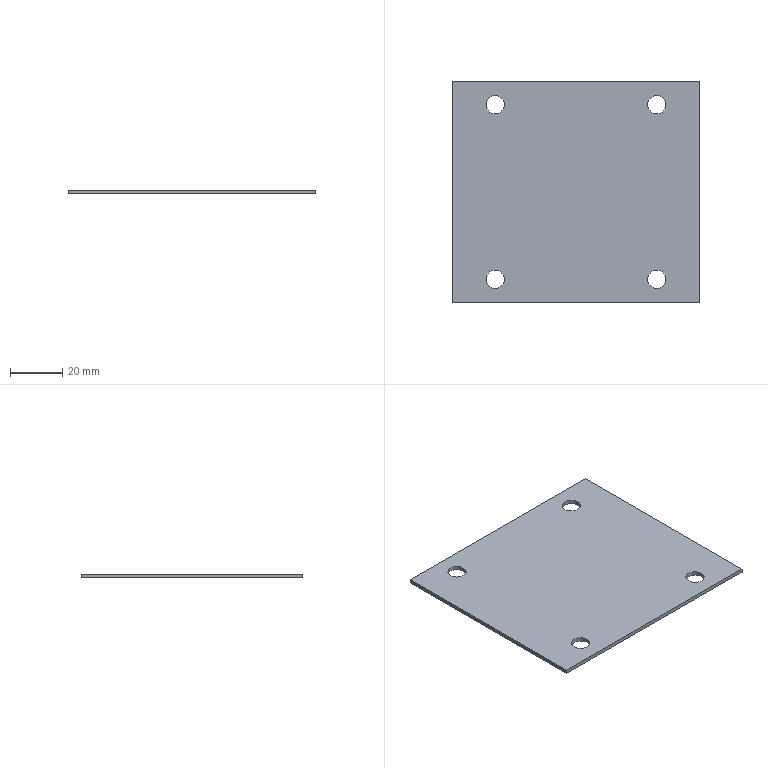Part | STEP file | GLSJ-10-46 | 1 solid | 14 faces | box 95 x 85 x 1.5 mm | volume 11882 mm3 | cylinder 8 | plane 6 | commonest cylinder face diameters 7 x8
STEP:
#1=CARTESIAN_POINT('',(0.,0.,0.));
#2=DIRECTION('',(0.,0.,1.));
#3=DIRECTION('',(1.,0.,0.));
#4=AXIS2_PLACEMENT_3D('',#1,#2,#3);
#5=CARTESIAN_POINT('',(-27.5,-33.5,0.));
#6=VERTEX_POINT('',#5);
#7=CARTESIAN_POINT('',(-27.5,-33.5,1.5));
#8=VERTEX_POINT('',#7);
#9=CARTESIAN_POINT('',(-27.5,-33.5,0.));
#10=DIRECTION('',(0.,0.,1.));
#11=VECTOR('',#10,1.);
#12=LINE('',#9,#11);
#13=CARTESIAN_POINT('',(-31.,-33.5,0.));
#14=DIRECTION('',(0.,0.,1.));
#15=DIRECTION('',(1.,0.,0.));
#16=AXIS2_PLACEMENT_3D('',#13,#14,#15);
#17=CYLINDRICAL_SURFACE('',#16,3.5);
#18=CARTESIAN_POINT('',(6.283,0.));
#19=DIRECTION('',(0.,1.));
#20=VECTOR('',#19,1.);
#21=LINE('',#18,#20);
#22=(GEOMETRIC_REPRESENTATION_CONTEXT(2)PARAMETRIC_REPRESENTATION_CONTEXT()REPRESENTATION_CONTEXT('',''));
#23=DEFINITIONAL_REPRESENTATION('',(#21),#22);
#24=PCURVE('',#17,#23);
#25=CARTESIAN_POINT('',(-31.,-33.5,0.));
#26=DIRECTION('',(0.,0.,1.));
#27=DIRECTION('',(1.,0.,0.));
#28=AXIS2_PLACEMENT_3D('',#25,#26,#27);
#29=CYLINDRICAL_SURFACE('',#28,3.5);
#30=CARTESIAN_POINT('',(0.,0.));
#31=DIRECTION('',(0.,1.));
#32=VECTOR('',#31,1.);
#33=LINE('',#30,#32);
#34=(GEOMETRIC_REPRESENTATION_CONTEXT(2)PARAMETRIC_REPRESENTATION_CONTEXT()REPRESENTATION_CONTEXT('',''));
#35=DEFINITIONAL_REPRESENTATION('',(#33),#34);
#36=PCURVE('',#29,#35);
#37=SURFACE_CURVE('',#12,(#24,#36),.PCURVE_S1.);
#38=EDGE_CURVE('',#6,#8,#37,.T.);
#39=ORIENTED_EDGE('',*,*,#38,.T.);
#40=CARTESIAN_POINT('',(-34.5,-33.5,1.5));
#41=VERTEX_POINT('',#40);
#42=CARTESIAN_POINT('',(-31.,-33.5,1.5));
#43=DIRECTION('',(0.,0.,1.));
#44=DIRECTION('',(-1.,0.,0.));
#45=AXIS2_PLACEMENT_3D('',#42,#43,#44);
#46=CIRCLE('',#45,3.5);
#47=CARTESIAN_POINT('',(3.142,1.5));
#48=DIRECTION('',(1.,0.));
#49=VECTOR('',#48,1.);
#50=LINE('',#47,#49);
#51=(GEOMETRIC_REPRESENTATION_CONTEXT(2)PARAMETRIC_REPRESENTATION_CONTEXT()REPRESENTATION_CONTEXT('',''));
#52=DEFINITIONAL_REPRESENTATION('',(#50),#51);
#53=PCURVE('',#17,#52);
#54=CARTESIAN_POINT('',(0.,0.,1.5));
#55=DIRECTION('',(0.,0.,-1.));
#56=DIRECTION('',(-1.,0.,0.));
#57=AXIS2_PLACEMENT_3D('',#54,#55,#56);
#58=PLANE('',#57);
#59=CARTESIAN_POINT('',(34.5,-33.5));
#60=CARTESIAN_POINT('',(34.5,-39.562));
#61=CARTESIAN_POINT('',(29.25,-36.531));
#62=CARTESIAN_POINT('',(24.,-33.5));
#63=CARTESIAN_POINT('',(29.25,-30.469));
#64=CARTESIAN_POINT('',(34.5,-27.438));
#65=CARTESIAN_POINT('',(34.5,-33.5));
#66=(BOUNDED_CURVE()B_SPLINE_CURVE(2,(#59,#60,#61,#62,#63,#64,#65),.UNSPECIFIED.,.T.,.F.)B_SPLINE_CURVE_WITH_KNOTS((1,2,2,2,2,1),(-2.094,0.,2.094,4.189,6.283,8.378),.UNSPECIFIED.)CURVE()GEOMETRIC_REPRESENTATION_ITEM()RATIONAL_B_SPLINE_CURVE((1.,0.5,1.,0.5,1.,0.5,1.))REPRESENTATION_ITEM(''));
#67=(GEOMETRIC_REPRESENTATION_CONTEXT(2)PARAMETRIC_REPRESENTATION_CONTEXT()REPRESENTATION_CONTEXT('',''));
#68=DEFINITIONAL_REPRESENTATION('',(#66),#67);
#69=PCURVE('',#58,#68);
#70=SURFACE_CURVE('',#46,(#53,#69),.PCURVE_S1.);
#71=EDGE_CURVE('',#41,#8,#70,.T.);
#72=ORIENTED_EDGE('',*,*,#71,.F.);
#73=CARTESIAN_POINT('',(-34.5,-33.5,0.));
#74=VERTEX_POINT('',#73);
#75=CARTESIAN_POINT('',(-34.5,-33.5,0.));
#76=DIRECTION('',(0.,0.,1.));
#77=VECTOR('',#76,1.);
#78=LINE('',#75,#77);
#79=CARTESIAN_POINT('',(3.142,0.));
#80=DIRECTION('',(0.,1.));
#81=VECTOR('',#80,1.);
#82=LINE('',#79,#81);
#83=(GEOMETRIC_REPRESENTATION_CONTEXT(2)PARAMETRIC_REPRESENTATION_CONTEXT()REPRESENTATION_CONTEXT('',''));
#84=DEFINITIONAL_REPRESENTATION('',(#82),#83);
#85=PCURVE('',#17,#84);
#86=CARTESIAN_POINT('',(3.142,0.));
#87=DIRECTION('',(0.,1.));
#88=VECTOR('',#87,1.);
#89=LINE('',#86,#88);
#90=(GEOMETRIC_REPRESENTATION_CONTEXT(2)PARAMETRIC_REPRESENTATION_CONTEXT()REPRESENTATION_CONTEXT('',''));
#91=DEFINITIONAL_REPRESENTATION('',(#89),#90);
#92=PCURVE('',#29,#91);
#93=SURFACE_CURVE('',#78,(#85,#92),.PCURVE_S1.);
#94=EDGE_CURVE('',#74,#41,#93,.T.);
#95=ORIENTED_EDGE('',*,*,#94,.F.);
#96=CARTESIAN_POINT('',(-31.,-33.5,0.));
#97=DIRECTION('',(0.,0.,1.));
#98=DIRECTION('',(-1.,0.,0.));
#99=AXIS2_PLACEMENT_3D('',#96,#97,#98);
#100=CIRCLE('',#99,3.5);
#101=CARTESIAN_POINT('',(3.142,0.));
#102=DIRECTION('',(1.,0.));
#103=VECTOR('',#102,1.);
#104=LINE('',#101,#103);
#105=(GEOMETRIC_REPRESENTATION_CONTEXT(2)PARAMETRIC_REPRESENTATION_CONTEXT()REPRESENTATION_CONTEXT('',''));
#106=DEFINITIONAL_REPRESENTATION('',(#104),#105);
#107=PCURVE('',#17,#106);
#108=CARTESIAN_POINT('',(0.,0.,0.));
#109=DIRECTION('',(0.,0.,-1.));
#110=DIRECTION('',(-1.,0.,0.));
#111=AXIS2_PLACEMENT_3D('',#108,#109,#110);
#112=PLANE('',#111);
#113=CARTESIAN_POINT('',(34.5,-33.5));
#114=CARTESIAN_POINT('',(34.5,-39.562));
#115=CARTESIAN_POINT('',(29.25,-36.531));
#116=CARTESIAN_POINT('',(24.,-33.5));
#117=CARTESIAN_POINT('',(29.25,-30.469));
#118=CARTESIAN_POINT('',(34.5,-27.438));
#119=CARTESIAN_POINT('',(34.5,-33.5));
#120=(BOUNDED_CURVE()B_SPLINE_CURVE(2,(#113,#114,#115,#116,#117,#118,#119),.UNSPECIFIED.,.T.,.F.)B_SPLINE_CURVE_WITH_KNOTS((1,2,2,2,2,1),(-2.094,0.,2.094,4.189,6.283,8.378),.UNSPECIFIED.)CURVE()GEOMETRIC_REPRESENTATION_ITEM()RATIONAL_B_SPLINE_CURVE((1.,0.5,1.,0.5,1.,0.5,1.))REPRESENTATION_ITEM(''));
#121=(GEOMETRIC_REPRESENTATION_CONTEXT(2)PARAMETRIC_REPRESENTATION_CONTEXT()REPRESENTATION_CONTEXT('',''));
#122=DEFINITIONAL_REPRESENTATION('',(#120),#121);
#123=PCURVE('',#112,#122);
#124=SURFACE_CURVE('',#100,(#107,#123),.PCURVE_S1.);
#125=EDGE_CURVE('',#74,#6,#124,.T.);
#126=ORIENTED_EDGE('',*,*,#125,.T.);
#127=EDGE_LOOP('',(#39,#72,#95,#126));
#128=FACE_BOUND('',#127,.F.);
#129=ADVANCED_FACE('',(#128),#17,.F.);
#130=CARTESIAN_POINT('',(34.5,-33.5,0.));
#131=VERTEX_POINT('',#130);
#132=CARTESIAN_POINT('',(34.5,-33.5,1.5));
#133=VERTEX_POINT('',#132);
#134=CARTESIAN_POINT('',(34.5,-33.5,0.));
#135=DIRECTION('',(0.,0.,1.));
#136=VECTOR('',#135,1.);
#137=LINE('',#134,#136);
#138=CARTESIAN_POINT('',(31.,-33.5,0.));
#139=DIRECTION('',(0.,0.,1.));
#140=DIRECTION('',(1.,0.,0.));
#141=AXIS2_PLACEMENT_3D('',#138,#139,#140);
#142=CYLINDRICAL_SURFACE('',#141,3.5);
#143=CARTESIAN_POINT('',(6.283,0.));
#144=DIRECTION('',(0.,1.));
#145=VECTOR('',#144,1.);
#146=LINE('',#143,#145);
#147=(GEOMETRIC_REPRESENTATION_CONTEXT(2)PARAMETRIC_REPRESENTATION_CONTEXT()REPRESENTATION_CONTEXT('',''));
#148=DEFINITIONAL_REPRESENTATION('',(#146),#147);
#149=PCURVE('',#142,#148);
#150=CARTESIAN_POINT('',(31.,-33.5,0.));
#151=DIRECTION('',(0.,0.,1.));
#152=DIRECTION('',(1.,0.,0.));
#153=AXIS2_PLACEMENT_3D('',#150,#151,#152);
#154=CYLINDRICAL_SURFACE('',#153,3.5);
#155=CARTESIAN_POINT('',(0.,0.));
#156=DIRECTION('',(0.,1.));
#157=VECTOR('',#156,1.);
#158=LINE('',#155,#157);
#159=(GEOMETRIC_REPRESENTATION_CONTEXT(2)PARAMETRIC_REPRESENTATION_CONTEXT()REPRESENTATION_CONTEXT('',''));
#160=DEFINITIONAL_REPRESENTATION('',(#158),#159);
#161=PCURVE('',#154,#160);
#162=SURFACE_CURVE('',#137,(#149,#161),.PCURVE_S1.);
#163=EDGE_CURVE('',#131,#133,#162,.T.);
#164=ORIENTED_EDGE('',*,*,#163,.T.);
#165=CARTESIAN_POINT('',(27.5,-33.5,1.5));
#166=VERTEX_POINT('',#165);
#167=CARTESIAN_POINT('',(31.,-33.5,1.5));
#168=DIRECTION('',(0.,0.,1.));
#169=DIRECTION('',(1.,0.,0.));
#170=AXIS2_PLACEMENT_3D('',#167,#168,#169);
#171=CIRCLE('',#170,3.5);
#172=CARTESIAN_POINT('',(0.,1.5));
#173=DIRECTION('',(1.,0.));
#174=VECTOR('',#173,1.);
#175=LINE('',#172,#174);
#176=(GEOMETRIC_REPRESENTATION_CONTEXT(2)PARAMETRIC_REPRESENTATION_CONTEXT()REPRESENTATION_CONTEXT('',''));
#177=DEFINITIONAL_REPRESENTATION('',(#175),#176);
#178=PCURVE('',#142,#177);
#179=CARTESIAN_POINT('',(-34.5,-33.5));
#180=CARTESIAN_POINT('',(-34.5,-27.438));
#181=CARTESIAN_POINT('',(-29.25,-30.469));
#182=CARTESIAN_POINT('',(-24.,-33.5));
#183=CARTESIAN_POINT('',(-29.25,-36.531));
#184=CARTESIAN_POINT('',(-34.5,-39.562));
#185=CARTESIAN_POINT('',(-34.5,-33.5));
#186=(BOUNDED_CURVE()B_SPLINE_CURVE(2,(#179,#180,#181,#182,#183,#184,#185),.UNSPECIFIED.,.T.,.F.)B_SPLINE_CURVE_WITH_KNOTS((1,2,2,2,2,1),(-2.094,0.,2.094,4.189,6.283,8.378),.UNSPECIFIED.)CURVE()GEOMETRIC_REPRESENTATION_ITEM()RATIONAL_B_SPLINE_CURVE((1.,0.5,1.,0.5,1.,0.5,1.))REPRESENTATION_ITEM(''));
#187=(GEOMETRIC_REPRESENTATION_CONTEXT(2)PARAMETRIC_REPRESENTATION_CONTEXT()REPRESENTATION_CONTEXT('',''));
#188=DEFINITIONAL_REPRESENTATION('',(#186),#187);
#189=PCURVE('',#58,#188);
#190=SURFACE_CURVE('',#171,(#178,#189),.PCURVE_S1.);
#191=EDGE_CURVE('',#166,#133,#190,.T.);
#192=ORIENTED_EDGE('',*,*,#191,.F.);
#193=CARTESIAN_POINT('',(27.5,-33.5,0.));
#194=VERTEX_POINT('',#193);
#195=CARTESIAN_POINT('',(27.5,-33.5,0.));
#196=DIRECTION('',(0.,0.,1.));
#197=VECTOR('',#196,1.);
#198=LINE('',#195,#197);
#199=CARTESIAN_POINT('',(3.142,0.));
#200=DIRECTION('',(0.,1.));
#201=VECTOR('',#200,1.);
#202=LINE('',#199,#201);
#203=(GEOMETRIC_REPRESENTATION_CONTEXT(2)PARAMETRIC_REPRESENTATION_CONTEXT()REPRESENTATION_CONTEXT('',''));
#204=DEFINITIONAL_REPRESENTATION('',(#202),#203);
#205=PCURVE('',#142,#204);
#206=CARTESIAN_POINT('',(3.142,0.));
#207=DIRECTION('',(0.,1.));
#208=VECTOR('',#207,1.);
#209=LINE('',#206,#208);
#210=(GEOMETRIC_REPRESENTATION_CONTEXT(2)PARAMETRIC_REPRESENTATION_CONTEXT()REPRESENTATION_CONTEXT('',''));
#211=DEFINITIONAL_REPRESENTATION('',(#209),#210);
#212=PCURVE('',#154,#211);
#213=SURFACE_CURVE('',#198,(#205,#212),.PCURVE_S1.);
#214=EDGE_CURVE('',#194,#166,#213,.T.);
#215=ORIENTED_EDGE('',*,*,#214,.F.);
#216=CARTESIAN_POINT('',(31.,-33.5,0.));
#217=DIRECTION('',(0.,0.,1.));
#218=DIRECTION('',(1.,0.,0.));
#219=AXIS2_PLACEMENT_3D('',#216,#217,#218);
#220=CIRCLE('',#219,3.5);
#221=CARTESIAN_POINT('',(0.,0.));
#222=DIRECTION('',(1.,0.));
#223=VECTOR('',#222,1.);
#224=LINE('',#221,#223);
#225=(GEOMETRIC_REPRESENTATION_CONTEXT(2)PARAMETRIC_REPRESENTATION_CONTEXT()REPRESENTATION_CONTEXT('',''));
#226=DEFINITIONAL_REPRESENTATION('',(#224),#225);
#227=PCURVE('',#142,#226);
#228=CARTESIAN_POINT('',(-34.5,-33.5));
#229=CARTESIAN_POINT('',(-34.5,-27.438));
#230=CARTESIAN_POINT('',(-29.25,-30.469));
#231=CARTESIAN_POINT('',(-24.,-33.5));
#232=CARTESIAN_POINT('',(-29.25,-36.531));
#233=CARTESIAN_POINT('',(-34.5,-39.562));
#234=CARTESIAN_POINT('',(-34.5,-33.5));
#235=(BOUNDED_CURVE()B_SPLINE_CURVE(2,(#228,#229,#230,#231,#232,#233,#234),.UNSPECIFIED.,.T.,.F.)B_SPLINE_CURVE_WITH_KNOTS((1,2,2,2,2,1),(-2.094,0.,2.094,4.189,6.283,8.378),.UNSPECIFIED.)CURVE()GEOMETRIC_REPRESENTATION_ITEM()RATIONAL_B_SPLINE_CURVE((1.,0.5,1.,0.5,1.,0.5,1.))REPRESENTATION_ITEM(''));
#236=(GEOMETRIC_REPRESENTATION_CONTEXT(2)PARAMETRIC_REPRESENTATION_CONTEXT()REPRESENTATION_CONTEXT('',''));
#237=DEFINITIONAL_REPRESENTATION('',(#235),#236);
#238=PCURVE('',#112,#237);
#239=SURFACE_CURVE('',#220,(#227,#238),.PCURVE_S1.);
#240=EDGE_CURVE('',#194,#131,#239,.T.);
#241=ORIENTED_EDGE('',*,*,#240,.T.);
#242=EDGE_LOOP('',(#164,#192,#215,#241));
#243=FACE_BOUND('',#242,.F.);
#244=ADVANCED_FACE('',(#243),#142,.F.);
#245=CARTESIAN_POINT('',(34.5,33.5,0.));
#246=VERTEX_POINT('',#245);
#247=CARTESIAN_POINT('',(34.5,33.5,1.5));
#248=VERTEX_POINT('',#247);
#249=CARTESIAN_POINT('',(34.5,33.5,0.));
#250=DIRECTION('',(0.,0.,1.));
#251=VECTOR('',#250,1.);
#252=LINE('',#249,#251);
#253=CARTESIAN_POINT('',(31.,33.5,0.));
#254=DIRECTION('',(0.,0.,1.));
#255=DIRECTION('',(1.,0.,0.));
#256=AXIS2_PLACEMENT_3D('',#253,#254,#255);
#257=CYLINDRICAL_SURFACE('',#256,3.5);
#258=CARTESIAN_POINT('',(6.283,0.));
#259=DIRECTION('',(0.,1.));
#260=VECTOR('',#259,1.);
#261=LINE('',#258,#260);
#262=(GEOMETRIC_REPRESENTATION_CONTEXT(2)PARAMETRIC_REPRESENTATION_CONTEXT()REPRESENTATION_CONTEXT('',''));
#263=DEFINITIONAL_REPRESENTATION('',(#261),#262);
#264=PCURVE('',#257,#263);
#265=CARTESIAN_POINT('',(31.,33.5,0.));
#266=DIRECTION('',(0.,0.,1.));
#267=DIRECTION('',(1.,0.,0.));
#268=AXIS2_PLACEMENT_3D('',#265,#266,#267);
#269=CYLINDRICAL_SURFACE('',#268,3.5);
#270=CARTESIAN_POINT('',(0.,0.));
#271=DIRECTION('',(0.,1.));
#272=VECTOR('',#271,1.);
#273=LINE('',#270,#272);
#274=(GEOMETRIC_REPRESENTATION_CONTEXT(2)PARAMETRIC_REPRESENTATION_CONTEXT()REPRESENTATION_CONTEXT('',''));
#275=DEFINITIONAL_REPRESENTATION('',(#273),#274);
#276=PCURVE('',#269,#275);
#277=SURFACE_CURVE('',#252,(#264,#276),.PCURVE_S1.);
#278=EDGE_CURVE('',#246,#248,#277,.T.);
#279=ORIENTED_EDGE('',*,*,#278,.T.);
#280=CARTESIAN_POINT('',(27.5,33.5,1.5));
#281=VERTEX_POINT('',#280);
#282=CARTESIAN_POINT('',(31.,33.5,1.5));
#283=DIRECTION('',(0.,0.,1.));
#284=DIRECTION('',(-1.,0.,0.));
#285=AXIS2_PLACEMENT_3D('',#282,#283,#284);
#286=CIRCLE('',#285,3.5);
#287=CARTESIAN_POINT('',(3.142,1.5));
#288=DIRECTION('',(1.,0.));
#289=VECTOR('',#288,1.);
#290=LINE('',#287,#289);
#291=(GEOMETRIC_REPRESENTATION_CONTEXT(2)PARAMETRIC_REPRESENTATION_CONTEXT()REPRESENTATION_CONTEXT('',''));
#292=DEFINITIONAL_REPRESENTATION('',(#290),#291);
#293=PCURVE('',#257,#292);
#294=CARTESIAN_POINT('',(-27.5,33.5));
#295=CARTESIAN_POINT('',(-27.5,27.438));
#296=CARTESIAN_POINT('',(-32.75,30.469));
#297=CARTESIAN_POINT('',(-38.,33.5));
#298=CARTESIAN_POINT('',(-32.75,36.531));
#299=CARTESIAN_POINT('',(-27.5,39.562));
#300=CARTESIAN_POINT('',(-27.5,33.5));
#301=(BOUNDED_CURVE()B_SPLINE_CURVE(2,(#294,#295,#296,#297,#298,#299,#300),.UNSPECIFIED.,.T.,.F.)B_SPLINE_CURVE_WITH_KNOTS((1,2,2,2,2,1),(-2.094,0.,2.094,4.189,6.283,8.378),.UNSPECIFIED.)CURVE()GEOMETRIC_REPRESENTATION_ITEM()RATIONAL_B_SPLINE_CURVE((1.,0.5,1.,0.5,1.,0.5,1.))REPRESENTATION_ITEM(''));
#302=(GEOMETRIC_REPRESENTATION_CONTEXT(2)PARAMETRIC_REPRESENTATION_CONTEXT()REPRESENTATION_CONTEXT('',''));
#303=DEFINITIONAL_REPRESENTATION('',(#301),#302);
#304=PCURVE('',#58,#303);
#305=SURFACE_CURVE('',#286,(#293,#304),.PCURVE_S1.);
#306=EDGE_CURVE('',#281,#248,#305,.T.);
#307=ORIENTED_EDGE('',*,*,#306,.F.);
#308=CARTESIAN_POINT('',(27.5,33.5,0.));
#309=VERTEX_POINT('',#308);
#310=CARTESIAN_POINT('',(27.5,33.5,0.));
#311=DIRECTION('',(0.,0.,1.));
#312=VECTOR('',#311,1.);
#313=LINE('',#310,#312);
#314=CARTESIAN_POINT('',(3.142,0.));
#315=DIRECTION('',(0.,1.));
#316=VECTOR('',#315,1.);
#317=LINE('',#314,#316);
#318=(GEOMETRIC_REPRESENTATION_CONTEXT(2)PARAMETRIC_REPRESENTATION_CONTEXT()REPRESENTATION_CONTEXT('',''));
#319=DEFINITIONAL_REPRESENTATION('',(#317),#318);
#320=PCURVE('',#257,#319);
#321=CARTESIAN_POINT('',(3.142,0.));
#322=DIRECTION('',(0.,1.));
#323=VECTOR('',#322,1.);
#324=LINE('',#321,#323);
#325=(GEOMETRIC_REPRESENTATION_CONTEXT(2)PARAMETRIC_REPRESENTATION_CONTEXT()REPRESENTATION_CONTEXT('',''));
#326=DEFINITIONAL_REPRESENTATION('',(#324),#325);
#327=PCURVE('',#269,#326);
#328=SURFACE_CURVE('',#313,(#320,#327),.PCURVE_S1.);
#329=EDGE_CURVE('',#309,#281,#328,.T.);
#330=ORIENTED_EDGE('',*,*,#329,.F.);
#331=CARTESIAN_POINT('',(31.,33.5,0.));
#332=DIRECTION('',(0.,0.,1.));
#333=DIRECTION('',(-1.,0.,0.));
#334=AXIS2_PLACEMENT_3D('',#331,#332,#333);
#335=CIRCLE('',#334,3.5);
#336=CARTESIAN_POINT('',(3.142,0.));
#337=DIRECTION('',(1.,0.));
#338=VECTOR('',#337,1.);
#339=LINE('',#336,#338);
#340=(GEOMETRIC_REPRESENTATION_CONTEXT(2)PARAMETRIC_REPRESENTATION_CONTEXT()REPRESENTATION_CONTEXT('',''));
#341=DEFINITIONAL_REPRESENTATION('',(#339),#340);
#342=PCURVE('',#257,#341);
#343=CARTESIAN_POINT('',(-27.5,33.5));
#344=CARTESIAN_POINT('',(-27.5,27.438));
#345=CARTESIAN_POINT('',(-32.75,30.469));
#346=CARTESIAN_POINT('',(-38.,33.5));
#347=CARTESIAN_POINT('',(-32.75,36.531));
#348=CARTESIAN_POINT('',(-27.5,39.562));
#349=CARTESIAN_POINT('',(-27.5,33.5));
#350=(BOUNDED_CURVE()B_SPLINE_CURVE(2,(#343,#344,#345,#346,#347,#348,#349),.UNSPECIFIED.,.T.,.F.)B_SPLINE_CURVE_WITH_KNOTS((1,2,2,2,2,1),(-2.094,0.,2.094,4.189,6.283,8.378),.UNSPECIFIED.)CURVE()GEOMETRIC_REPRESENTATION_ITEM()RATIONAL_B_SPLINE_CURVE((1.,0.5,1.,0.5,1.,0.5,1.))REPRESENTATION_ITEM(''));
#351=(GEOMETRIC_REPRESENTATION_CONTEXT(2)PARAMETRIC_REPRESENTATION_CONTEXT()REPRESENTATION_CONTEXT('',''));
#352=DEFINITIONAL_REPRESENTATION('',(#350),#351);
#353=PCURVE('',#112,#352);
#354=SURFACE_CURVE('',#335,(#342,#353),.PCURVE_S1.);
#355=EDGE_CURVE('',#309,#246,#354,.T.);
#356=ORIENTED_EDGE('',*,*,#355,.T.);
#357=EDGE_LOOP('',(#279,#307,#330,#356));
#358=FACE_BOUND('',#357,.F.);
#359=ADVANCED_FACE('',(#358),#257,.F.);
#360=CARTESIAN_POINT('',(-27.5,33.5,0.));
#361=VERTEX_POINT('',#360);
#362=CARTESIAN_POINT('',(-27.5,33.5,1.5));
#363=VERTEX_POINT('',#362);
#364=CARTESIAN_POINT('',(-27.5,33.5,0.));
#365=DIRECTION('',(0.,0.,1.));
#366=VECTOR('',#365,1.);
#367=LINE('',#364,#366);
#368=CARTESIAN_POINT('',(-31.,33.5,0.));
#369=DIRECTION('',(0.,0.,1.));
#370=DIRECTION('',(1.,0.,0.));
#371=AXIS2_PLACEMENT_3D('',#368,#369,#370);
#372=CYLINDRICAL_SURFACE('',#371,3.5);
#373=CARTESIAN_POINT('',(6.283,0.));
#374=DIRECTION('',(0.,1.));
#375=VECTOR('',#374,1.);
#376=LINE('',#373,#375);
#377=(GEOMETRIC_REPRESENTATION_CONTEXT(2)PARAMETRIC_REPRESENTATION_CONTEXT()REPRESENTATION_CONTEXT('',''));
#378=DEFINITIONAL_REPRESENTATION('',(#376),#377);
#379=PCURVE('',#372,#378);
#380=CARTESIAN_POINT('',(-31.,33.5,0.));
#381=DIRECTION('',(0.,0.,1.));
#382=DIRECTION('',(1.,0.,0.));
#383=AXIS2_PLACEMENT_3D('',#380,#381,#382);
#384=CYLINDRICAL_SURFACE('',#383,3.5);
#385=CARTESIAN_POINT('',(0.,0.));
#386=DIRECTION('',(0.,1.));
#387=VECTOR('',#386,1.);
#388=LINE('',#385,#387);
#389=(GEOMETRIC_REPRESENTATION_CONTEXT(2)PARAMETRIC_REPRESENTATION_CONTEXT()REPRESENTATION_CONTEXT('',''));
#390=DEFINITIONAL_REPRESENTATION('',(#388),#389);
#391=PCURVE('',#384,#390);
#392=SURFACE_CURVE('',#367,(#379,#391),.PCURVE_S1.);
#393=EDGE_CURVE('',#361,#363,#392,.T.);
#394=ORIENTED_EDGE('',*,*,#393,.T.);
#395=CARTESIAN_POINT('',(-34.5,33.5,1.5));
#396=VERTEX_POINT('',#395);
#397=CARTESIAN_POINT('',(-31.,33.5,1.5));
#398=DIRECTION('',(0.,0.,1.));
#399=DIRECTION('',(1.,0.,0.));
#400=AXIS2_PLACEMENT_3D('',#397,#398,#399);
#401=CIRCLE('',#400,3.5);
#402=CARTESIAN_POINT('',(0.,1.5));
#403=DIRECTION('',(1.,0.));
#404=VECTOR('',#403,1.);
#405=LINE('',#402,#404);
#406=(GEOMETRIC_REPRESENTATION_CONTEXT(2)PARAMETRIC_REPRESENTATION_CONTEXT()REPRESENTATION_CONTEXT('',''));
#407=DEFINITIONAL_REPRESENTATION('',(#405),#406);
#408=PCURVE('',#372,#407);
#409=CARTESIAN_POINT('',(27.5,33.5));
#410=CARTESIAN_POINT('',(27.5,39.562));
#411=CARTESIAN_POINT('',(32.75,36.531));
#412=CARTESIAN_POINT('',(38.,33.5));
#413=CARTESIAN_POINT('',(32.75,30.469));
#414=CARTESIAN_POINT('',(27.5,27.438));
#415=CARTESIAN_POINT('',(27.5,33.5));
#416=(BOUNDED_CURVE()B_SPLINE_CURVE(2,(#409,#410,#411,#412,#413,#414,#415),.UNSPECIFIED.,.T.,.F.)B_SPLINE_CURVE_WITH_KNOTS((1,2,2,2,2,1),(-2.094,0.,2.094,4.189,6.283,8.378),.UNSPECIFIED.)CURVE()GEOMETRIC_REPRESENTATION_ITEM()RATIONAL_B_SPLINE_CURVE((1.,0.5,1.,0.5,1.,0.5,1.))REPRESENTATION_ITEM(''));
#417=(GEOMETRIC_REPRESENTATION_CONTEXT(2)PARAMETRIC_REPRESENTATION_CONTEXT()REPRESENTATION_CONTEXT('',''));
#418=DEFINITIONAL_REPRESENTATION('',(#416),#417);
#419=PCURVE('',#58,#418);
#420=SURFACE_CURVE('',#401,(#408,#419),.PCURVE_S1.);
#421=EDGE_CURVE('',#396,#363,#420,.T.);
#422=ORIENTED_EDGE('',*,*,#421,.F.);
#423=CARTESIAN_POINT('',(-34.5,33.5,0.));
#424=VERTEX_POINT('',#423);
#425=CARTESIAN_POINT('',(-34.5,33.5,0.));
#426=DIRECTION('',(0.,0.,1.));
#427=VECTOR('',#426,1.);
#428=LINE('',#425,#427);
#429=CARTESIAN_POINT('',(3.142,0.));
#430=DIRECTION('',(0.,1.));
#431=VECTOR('',#430,1.);
#432=LINE('',#429,#431);
#433=(GEOMETRIC_REPRESENTATION_CONTEXT(2)PARAMETRIC_REPRESENTATION_CONTEXT()REPRESENTATION_CONTEXT('',''));
#434=DEFINITIONAL_REPRESENTATION('',(#432),#433);
#435=PCURVE('',#372,#434);
#436=CARTESIAN_POINT('',(3.142,0.));
#437=DIRECTION('',(0.,1.));
#438=VECTOR('',#437,1.);
#439=LINE('',#436,#438);
#440=(GEOMETRIC_REPRESENTATION_CONTEXT(2)PARAMETRIC_REPRESENTATION_CONTEXT()REPRESENTATION_CONTEXT('',''));
#441=DEFINITIONAL_REPRESENTATION('',(#439),#440);
#442=PCURVE('',#384,#441);
#443=SURFACE_CURVE('',#428,(#435,#442),.PCURVE_S1.);
#444=EDGE_CURVE('',#424,#396,#443,.T.);
#445=ORIENTED_EDGE('',*,*,#444,.F.);
#446=CARTESIAN_POINT('',(-31.,33.5,0.));
#447=DIRECTION('',(0.,0.,1.));
#448=DIRECTION('',(1.,0.,0.));
#449=AXIS2_PLACEMENT_3D('',#446,#447,#448);
#450=CIRCLE('',#449,3.5);
#451=CARTESIAN_POINT('',(0.,0.));
#452=DIRECTION('',(1.,0.));
#453=VECTOR('',#452,1.);
#454=LINE('',#451,#453);
#455=(GEOMETRIC_REPRESENTATION_CONTEXT(2)PARAMETRIC_REPRESENTATION_CONTEXT()REPRESENTATION_CONTEXT('',''));
#456=DEFINITIONAL_REPRESENTATION('',(#454),#455);
#457=PCURVE('',#372,#456);
#458=CARTESIAN_POINT('',(27.5,33.5));
#459=CARTESIAN_POINT('',(27.5,39.562));
#460=CARTESIAN_POINT('',(32.75,36.531));
#461=CARTESIAN_POINT('',(38.,33.5));
#462=CARTESIAN_POINT('',(32.75,30.469));
#463=CARTESIAN_POINT('',(27.5,27.438));
#464=CARTESIAN_POINT('',(27.5,33.5));
#465=(BOUNDED_CURVE()B_SPLINE_CURVE(2,(#458,#459,#460,#461,#462,#463,#464),.UNSPECIFIED.,.T.,.F.)B_SPLINE_CURVE_WITH_KNOTS((1,2,2,2,2,1),(-2.094,0.,2.094,4.189,6.283,8.378),.UNSPECIFIED.)CURVE()GEOMETRIC_REPRESENTATION_ITEM()RATIONAL_B_SPLINE_CURVE((1.,0.5,1.,0.5,1.,0.5,1.))REPRESENTATION_ITEM(''));
#466=(GEOMETRIC_REPRESENTATION_CONTEXT(2)PARAMETRIC_REPRESENTATION_CONTEXT()REPRESENTATION_CONTEXT('',''));
#467=DEFINITIONAL_REPRESENTATION('',(#465),#466);
#468=PCURVE('',#112,#467);
#469=SURFACE_CURVE('',#450,(#457,#468),.PCURVE_S1.);
#470=EDGE_CURVE('',#424,#361,#469,.T.);
#471=ORIENTED_EDGE('',*,*,#470,.T.);
#472=EDGE_LOOP('',(#394,#422,#445,#471));
#473=FACE_BOUND('',#472,.F.);
#474=ADVANCED_FACE('',(#473),#372,.F.);
#475=CARTESIAN_POINT('',(-47.5,42.5,0.));
#476=VERTEX_POINT('',#475);
#477=CARTESIAN_POINT('',(-47.5,-42.5,0.));
#478=VERTEX_POINT('',#477);
#479=CARTESIAN_POINT('',(-47.5,42.5,0.));
#480=DIRECTION('',(0.,-1.,0.));
#481=VECTOR('',#480,1.);
#482=LINE('',#479,#481);
#483=CARTESIAN_POINT('',(-47.5,42.5,1.5));
#484=DIRECTION('',(1.,0.,0.));
#485=DIRECTION('',(0.,1.,0.));
#486=AXIS2_PLACEMENT_3D('',#483,#484,#485);
#487=PLANE('',#486);
#488=CARTESIAN_POINT('',(0.,-1.5));
#489=DIRECTION('',(-1.,0.));
#490=VECTOR('',#489,1.);
#491=LINE('',#488,#490);
#492=(GEOMETRIC_REPRESENTATION_CONTEXT(2)PARAMETRIC_REPRESENTATION_CONTEXT()REPRESENTATION_CONTEXT('',''));
#493=DEFINITIONAL_REPRESENTATION('',(#491),#492);
#494=PCURVE('',#487,#493);
#495=CARTESIAN_POINT('',(47.5,42.5));
#496=DIRECTION('',(0.,-1.));
#497=VECTOR('',#496,1.);
#498=LINE('',#495,#497);
#499=(GEOMETRIC_REPRESENTATION_CONTEXT(2)PARAMETRIC_REPRESENTATION_CONTEXT()REPRESENTATION_CONTEXT('',''));
#500=DEFINITIONAL_REPRESENTATION('',(#498),#499);
#501=PCURVE('',#112,#500);
#502=SURFACE_CURVE('',#482,(#494,#501),.PCURVE_S1.);
#503=EDGE_CURVE('',#476,#478,#502,.T.);
#504=ORIENTED_EDGE('',*,*,#503,.T.);
#505=CARTESIAN_POINT('',(-47.5,-42.5,1.5));
#506=VERTEX_POINT('',#505);
#507=CARTESIAN_POINT('',(-47.5,-42.5,1.5));
#508=DIRECTION('',(0.,0.,-1.));
#509=VECTOR('',#508,1.);
#510=LINE('',#507,#509);
#511=CARTESIAN_POINT('',(-85.,0.));
#512=DIRECTION('',(0.,-1.));
#513=VECTOR('',#512,1.);
#514=LINE('',#511,#513);
#515=(GEOMETRIC_REPRESENTATION_CONTEXT(2)PARAMETRIC_REPRESENTATION_CONTEXT()REPRESENTATION_CONTEXT('',''));
#516=DEFINITIONAL_REPRESENTATION('',(#514),#515);
#517=PCURVE('',#487,#516);
#518=CARTESIAN_POINT('',(47.5,-42.5,1.5));
#519=DIRECTION('',(0.,1.,0.));
#520=DIRECTION('',(-1.,0.,0.));
#521=AXIS2_PLACEMENT_3D('',#518,#519,#520);
#522=PLANE('',#521);
#523=CARTESIAN_POINT('',(95.,0.));
#524=DIRECTION('',(0.,-1.));
#525=VECTOR('',#524,1.);
#526=LINE('',#523,#525);
#527=(GEOMETRIC_REPRESENTATION_CONTEXT(2)PARAMETRIC_REPRESENTATION_CONTEXT()REPRESENTATION_CONTEXT('',''));
#528=DEFINITIONAL_REPRESENTATION('',(#526),#527);
#529=PCURVE('',#522,#528);
#530=SURFACE_CURVE('',#510,(#517,#529),.PCURVE_S1.);
#531=EDGE_CURVE('',#506,#478,#530,.T.);
#532=ORIENTED_EDGE('',*,*,#531,.F.);
#533=CARTESIAN_POINT('',(-47.5,42.5,1.5));
#534=VERTEX_POINT('',#533);
#535=CARTESIAN_POINT('',(-47.5,42.5,1.5));
#536=DIRECTION('',(0.,-1.,0.));
#537=VECTOR('',#536,1.);
#538=LINE('',#535,#537);
#539=CARTESIAN_POINT('',(0.,0.));
#540=DIRECTION('',(-1.,0.));
#541=VECTOR('',#540,1.);
#542=LINE('',#539,#541);
#543=(GEOMETRIC_REPRESENTATION_CONTEXT(2)PARAMETRIC_REPRESENTATION_CONTEXT()REPRESENTATION_CONTEXT('',''));
#544=DEFINITIONAL_REPRESENTATION('',(#542),#543);
#545=PCURVE('',#487,#544);
#546=CARTESIAN_POINT('',(47.5,42.5));
#547=DIRECTION('',(0.,-1.));
#548=VECTOR('',#547,1.);
#549=LINE('',#546,#548);
#550=(GEOMETRIC_REPRESENTATION_CONTEXT(2)PARAMETRIC_REPRESENTATION_CONTEXT()REPRESENTATION_CONTEXT('',''));
#551=DEFINITIONAL_REPRESENTATION('',(#549),#550);
#552=PCURVE('',#58,#551);
#553=SURFACE_CURVE('',#538,(#545,#552),.PCURVE_S1.);
#554=EDGE_CURVE('',#534,#506,#553,.T.);
#555=ORIENTED_EDGE('',*,*,#554,.F.);
#556=CARTESIAN_POINT('',(-47.5,42.5,1.5));
#557=DIRECTION('',(0.,0.,-1.));
#558=VECTOR('',#557,1.);
#559=LINE('',#556,#558);
#560=CARTESIAN_POINT('',(0.,0.));
#561=DIRECTION('',(0.,-1.));
#562=VECTOR('',#561,1.);
#563=LINE('',#560,#562);
#564=(GEOMETRIC_REPRESENTATION_CONTEXT(2)PARAMETRIC_REPRESENTATION_CONTEXT()REPRESENTATION_CONTEXT('',''));
#565=DEFINITIONAL_REPRESENTATION('',(#563),#564);
#566=PCURVE('',#487,#565);
#567=CARTESIAN_POINT('',(47.5,42.5,1.5));
#568=DIRECTION('',(0.,-1.,0.));
#569=DIRECTION('',(1.,0.,0.));
#570=AXIS2_PLACEMENT_3D('',#567,#568,#569);
#571=PLANE('',#570);
#572=CARTESIAN_POINT('',(-95.,0.));
#573=DIRECTION('',(0.,-1.));
#574=VECTOR('',#573,1.);
#575=LINE('',#572,#574);
#576=(GEOMETRIC_REPRESENTATION_CONTEXT(2)PARAMETRIC_REPRESENTATION_CONTEXT()REPRESENTATION_CONTEXT('',''));
#577=DEFINITIONAL_REPRESENTATION('',(#575),#576);
#578=PCURVE('',#571,#577);
#579=SURFACE_CURVE('',#559,(#566,#578),.PCURVE_S1.);
#580=EDGE_CURVE('',#534,#476,#579,.T.);
#581=ORIENTED_EDGE('',*,*,#580,.T.);
#582=EDGE_LOOP('',(#504,#532,#555,#581));
#583=FACE_BOUND('',#582,.T.);
#584=ADVANCED_FACE('',(#583),#487,.F.);
#585=CARTESIAN_POINT('',(47.5,-42.5,0.));
#586=VERTEX_POINT('',#585);
#587=CARTESIAN_POINT('',(47.5,-42.5,0.));
#588=DIRECTION('',(1.,0.,0.));
#589=VECTOR('',#588,1.);
#590=LINE('',#587,#589);
#591=CARTESIAN_POINT('',(0.,-1.5));
#592=DIRECTION('',(-1.,0.));
#593=VECTOR('',#592,1.);
#594=LINE('',#591,#593);
#595=(GEOMETRIC_REPRESENTATION_CONTEXT(2)PARAMETRIC_REPRESENTATION_CONTEXT()REPRESENTATION_CONTEXT('',''));
#596=DEFINITIONAL_REPRESENTATION('',(#594),#595);
#597=PCURVE('',#522,#596);
#598=CARTESIAN_POINT('',(-47.5,-42.5));
#599=DIRECTION('',(-1.,0.));
#600=VECTOR('',#599,1.);
#601=LINE('',#598,#600);
#602=(GEOMETRIC_REPRESENTATION_CONTEXT(2)PARAMETRIC_REPRESENTATION_CONTEXT()REPRESENTATION_CONTEXT('',''));
#603=DEFINITIONAL_REPRESENTATION('',(#601),#602);
#604=PCURVE('',#112,#603);
#605=SURFACE_CURVE('',#590,(#597,#604),.PCURVE_S1.);
#606=EDGE_CURVE('',#478,#586,#605,.T.);
#607=ORIENTED_EDGE('',*,*,#606,.T.);
#608=CARTESIAN_POINT('',(47.5,-42.5,1.5));
#609=VERTEX_POINT('',#608);
#610=CARTESIAN_POINT('',(47.5,-42.5,1.5));
#611=DIRECTION('',(0.,0.,-1.));
#612=VECTOR('',#611,1.);
#613=LINE('',#610,#612);
#614=CARTESIAN_POINT('',(0.,0.));
#615=DIRECTION('',(0.,-1.));
#616=VECTOR('',#615,1.);
#617=LINE('',#614,#616);
#618=(GEOMETRIC_REPRESENTATION_CONTEXT(2)PARAMETRIC_REPRESENTATION_CONTEXT()REPRESENTATION_CONTEXT('',''));
#619=DEFINITIONAL_REPRESENTATION('',(#617),#618);
#620=PCURVE('',#522,#619);
#621=CARTESIAN_POINT('',(47.5,42.5,1.5));
#622=DIRECTION('',(-1.,0.,0.));
#623=DIRECTION('',(0.,-1.,0.));
#624=AXIS2_PLACEMENT_3D('',#621,#622,#623);
#625=PLANE('',#624);
#626=CARTESIAN_POINT('',(85.,0.));
#627=DIRECTION('',(0.,-1.));
#628=VECTOR('',#627,1.);
#629=LINE('',#626,#628);
#630=(GEOMETRIC_REPRESENTATION_CONTEXT(2)PARAMETRIC_REPRESENTATION_CONTEXT()REPRESENTATION_CONTEXT('',''));
#631=DEFINITIONAL_REPRESENTATION('',(#629),#630);
#632=PCURVE('',#625,#631);
#633=SURFACE_CURVE('',#613,(#620,#632),.PCURVE_S1.);
#634=EDGE_CURVE('',#609,#586,#633,.T.);
#635=ORIENTED_EDGE('',*,*,#634,.F.);
#636=CARTESIAN_POINT('',(47.5,-42.5,1.5));
#637=DIRECTION('',(1.,0.,0.));
#638=VECTOR('',#637,1.);
#639=LINE('',#636,#638);
#640=CARTESIAN_POINT('',(0.,0.));
#641=DIRECTION('',(-1.,0.));
#642=VECTOR('',#641,1.);
#643=LINE('',#640,#642);
#644=(GEOMETRIC_REPRESENTATION_CONTEXT(2)PARAMETRIC_REPRESENTATION_CONTEXT()REPRESENTATION_CONTEXT('',''));
#645=DEFINITIONAL_REPRESENTATION('',(#643),#644);
#646=PCURVE('',#522,#645);
#647=CARTESIAN_POINT('',(-47.5,-42.5));
#648=DIRECTION('',(-1.,0.));
#649=VECTOR('',#648,1.);
#650=LINE('',#647,#649);
#651=(GEOMETRIC_REPRESENTATION_CONTEXT(2)PARAMETRIC_REPRESENTATION_CONTEXT()REPRESENTATION_CONTEXT('',''));
#652=DEFINITIONAL_REPRESENTATION('',(#650),#651);
#653=PCURVE('',#58,#652);
#654=SURFACE_CURVE('',#639,(#646,#653),.PCURVE_S1.);
#655=EDGE_CURVE('',#506,#609,#654,.T.);
#656=ORIENTED_EDGE('',*,*,#655,.F.);
#657=ORIENTED_EDGE('',*,*,#531,.T.);
#658=EDGE_LOOP('',(#607,#635,#656,#657));
#659=FACE_BOUND('',#658,.T.);
#660=ADVANCED_FACE('',(#659),#522,.F.);
#661=CARTESIAN_POINT('',(47.5,42.5,0.));
#662=VERTEX_POINT('',#661);
#663=CARTESIAN_POINT('',(47.5,42.5,0.));
#664=DIRECTION('',(0.,1.,0.));
#665=VECTOR('',#664,1.);
#666=LINE('',#663,#665);
#667=CARTESIAN_POINT('',(0.,-1.5));
#668=DIRECTION('',(-1.,0.));
#669=VECTOR('',#668,1.);
#670=LINE('',#667,#669);
#671=(GEOMETRIC_REPRESENTATION_CONTEXT(2)PARAMETRIC_REPRESENTATION_CONTEXT()REPRESENTATION_CONTEXT('',''));
#672=DEFINITIONAL_REPRESENTATION('',(#670),#671);
#673=PCURVE('',#625,#672);
#674=CARTESIAN_POINT('',(-47.5,42.5));
#675=DIRECTION('',(0.,1.));
#676=VECTOR('',#675,1.);
#677=LINE('',#674,#676);
#678=(GEOMETRIC_REPRESENTATION_CONTEXT(2)PARAMETRIC_REPRESENTATION_CONTEXT()REPRESENTATION_CONTEXT('',''));
#679=DEFINITIONAL_REPRESENTATION('',(#677),#678);
#680=PCURVE('',#112,#679);
#681=SURFACE_CURVE('',#666,(#673,#680),.PCURVE_S1.);
#682=EDGE_CURVE('',#586,#662,#681,.T.);
#683=ORIENTED_EDGE('',*,*,#682,.T.);
#684=CARTESIAN_POINT('',(47.5,42.5,1.5));
#685=VERTEX_POINT('',#684);
#686=CARTESIAN_POINT('',(47.5,42.5,1.5));
#687=DIRECTION('',(0.,0.,-1.));
#688=VECTOR('',#687,1.);
#689=LINE('',#686,#688);
#690=CARTESIAN_POINT('',(0.,0.));
#691=DIRECTION('',(0.,-1.));
#692=VECTOR('',#691,1.);
#693=LINE('',#690,#692);
#694=(GEOMETRIC_REPRESENTATION_CONTEXT(2)PARAMETRIC_REPRESENTATION_CONTEXT()REPRESENTATION_CONTEXT('',''));
#695=DEFINITIONAL_REPRESENTATION('',(#693),#694);
#696=PCURVE('',#625,#695);
#697=CARTESIAN_POINT('',(0.,0.));
#698=DIRECTION('',(0.,-1.));
#699=VECTOR('',#698,1.);
#700=LINE('',#697,#699);
#701=(GEOMETRIC_REPRESENTATION_CONTEXT(2)PARAMETRIC_REPRESENTATION_CONTEXT()REPRESENTATION_CONTEXT('',''));
#702=DEFINITIONAL_REPRESENTATION('',(#700),#701);
#703=PCURVE('',#571,#702);
#704=SURFACE_CURVE('',#689,(#696,#703),.PCURVE_S1.);
#705=EDGE_CURVE('',#685,#662,#704,.T.);
#706=ORIENTED_EDGE('',*,*,#705,.F.);
#707=CARTESIAN_POINT('',(47.5,42.5,1.5));
#708=DIRECTION('',(0.,1.,0.));
#709=VECTOR('',#708,1.);
#710=LINE('',#707,#709);
#711=CARTESIAN_POINT('',(0.,0.));
#712=DIRECTION('',(-1.,0.));
#713=VECTOR('',#712,1.);
#714=LINE('',#711,#713);
#715=(GEOMETRIC_REPRESENTATION_CONTEXT(2)PARAMETRIC_REPRESENTATION_CONTEXT()REPRESENTATION_CONTEXT('',''));
#716=DEFINITIONAL_REPRESENTATION('',(#714),#715);
#717=PCURVE('',#625,#716);
#718=CARTESIAN_POINT('',(-47.5,42.5));
#719=DIRECTION('',(0.,1.));
#720=VECTOR('',#719,1.);
#721=LINE('',#718,#720);
#722=(GEOMETRIC_REPRESENTATION_CONTEXT(2)PARAMETRIC_REPRESENTATION_CONTEXT()REPRESENTATION_CONTEXT('',''));
#723=DEFINITIONAL_REPRESENTATION('',(#721),#722);
#724=PCURVE('',#58,#723);
#725=SURFACE_CURVE('',#710,(#717,#724),.PCURVE_S1.);
#726=EDGE_CURVE('',#609,#685,#725,.T.);
#727=ORIENTED_EDGE('',*,*,#726,.F.);
#728=ORIENTED_EDGE('',*,*,#634,.T.);
#729=EDGE_LOOP('',(#683,#706,#727,#728));
#730=FACE_BOUND('',#729,.T.);
#731=ADVANCED_FACE('',(#730),#625,.F.);
#732=CARTESIAN_POINT('',(47.5,42.5,0.));
#733=DIRECTION('',(-1.,0.,0.));
#734=VECTOR('',#733,1.);
#735=LINE('',#732,#734);
#736=CARTESIAN_POINT('',(0.,-1.5));
#737=DIRECTION('',(-1.,0.));
#738=VECTOR('',#737,1.);
#739=LINE('',#736,#738);
#740=(GEOMETRIC_REPRESENTATION_CONTEXT(2)PARAMETRIC_REPRESENTATION_CONTEXT()REPRESENTATION_CONTEXT('',''));
#741=DEFINITIONAL_REPRESENTATION('',(#739),#740);
#742=PCURVE('',#571,#741);
#743=CARTESIAN_POINT('',(-47.5,42.5));
#744=DIRECTION('',(1.,0.));
#745=VECTOR('',#744,1.);
#746=LINE('',#743,#745);
#747=(GEOMETRIC_REPRESENTATION_CONTEXT(2)PARAMETRIC_REPRESENTATION_CONTEXT()REPRESENTATION_CONTEXT('',''));
#748=DEFINITIONAL_REPRESENTATION('',(#746),#747);
#749=PCURVE('',#112,#748);
#750=SURFACE_CURVE('',#735,(#742,#749),.PCURVE_S1.);
#751=EDGE_CURVE('',#662,#476,#750,.T.);
#752=ORIENTED_EDGE('',*,*,#751,.T.);
#753=ORIENTED_EDGE('',*,*,#580,.F.);
#754=CARTESIAN_POINT('',(47.5,42.5,1.5));
#755=DIRECTION('',(-1.,0.,0.));
#756=VECTOR('',#755,1.);
#757=LINE('',#754,#756);
#758=CARTESIAN_POINT('',(0.,0.));
#759=DIRECTION('',(-1.,0.));
#760=VECTOR('',#759,1.);
#761=LINE('',#758,#760);
#762=(GEOMETRIC_REPRESENTATION_CONTEXT(2)PARAMETRIC_REPRESENTATION_CONTEXT()REPRESENTATION_CONTEXT('',''));
#763=DEFINITIONAL_REPRESENTATION('',(#761),#762);
#764=PCURVE('',#571,#763);
#765=CARTESIAN_POINT('',(-47.5,42.5));
#766=DIRECTION('',(1.,0.));
#767=VECTOR('',#766,1.);
#768=LINE('',#765,#767);
#769=(GEOMETRIC_REPRESENTATION_CONTEXT(2)PARAMETRIC_REPRESENTATION_CONTEXT()REPRESENTATION_CONTEXT('',''));
#770=DEFINITIONAL_REPRESENTATION('',(#768),#769);
#771=PCURVE('',#58,#770);
#772=SURFACE_CURVE('',#757,(#764,#771),.PCURVE_S1.);
#773=EDGE_CURVE('',#685,#534,#772,.T.);
#774=ORIENTED_EDGE('',*,*,#773,.F.);
#775=ORIENTED_EDGE('',*,*,#705,.T.);
#776=EDGE_LOOP('',(#752,#753,#774,#775));
#777=FACE_BOUND('',#776,.T.);
#778=ADVANCED_FACE('',(#777),#571,.F.);
#779=CARTESIAN_POINT('',(-31.,-33.5,1.5));
#780=DIRECTION('',(0.,0.,1.));
#781=DIRECTION('',(-1.,0.,0.));
#782=AXIS2_PLACEMENT_3D('',#779,#780,#781);
#783=CIRCLE('',#782,3.5);
#784=CARTESIAN_POINT('',(34.5,-33.5));
#785=CARTESIAN_POINT('',(34.5,-39.562));
#786=CARTESIAN_POINT('',(29.25,-36.531));
#787=CARTESIAN_POINT('',(24.,-33.5));
#788=CARTESIAN_POINT('',(29.25,-30.469));
#789=CARTESIAN_POINT('',(34.5,-27.438));
#790=CARTESIAN_POINT('',(34.5,-33.5));
#791=(BOUNDED_CURVE()B_SPLINE_CURVE(2,(#784,#785,#786,#787,#788,#789,#790),.UNSPECIFIED.,.T.,.F.)B_SPLINE_CURVE_WITH_KNOTS((1,2,2,2,2,1),(-2.094,0.,2.094,4.189,6.283,8.378),.UNSPECIFIED.)CURVE()GEOMETRIC_REPRESENTATION_ITEM()RATIONAL_B_SPLINE_CURVE((1.,0.5,1.,0.5,1.,0.5,1.))REPRESENTATION_ITEM(''));
#792=(GEOMETRIC_REPRESENTATION_CONTEXT(2)PARAMETRIC_REPRESENTATION_CONTEXT()REPRESENTATION_CONTEXT('',''));
#793=DEFINITIONAL_REPRESENTATION('',(#791),#792);
#794=PCURVE('',#58,#793);
#795=CARTESIAN_POINT('',(-3.142,1.5));
#796=DIRECTION('',(1.,0.));
#797=VECTOR('',#796,1.);
#798=LINE('',#795,#797);
#799=(GEOMETRIC_REPRESENTATION_CONTEXT(2)PARAMETRIC_REPRESENTATION_CONTEXT()REPRESENTATION_CONTEXT('',''));
#800=DEFINITIONAL_REPRESENTATION('',(#798),#799);
#801=PCURVE('',#29,#800);
#802=SURFACE_CURVE('',#783,(#794,#801),.PCURVE_S1.);
#803=EDGE_CURVE('',#8,#41,#802,.T.);
#804=ORIENTED_EDGE('',*,*,#803,.F.);
#805=ORIENTED_EDGE('',*,*,#71,.F.);
#806=EDGE_LOOP('',(#804,#805));
#807=FACE_BOUND('',#806,.T.);
#808=CARTESIAN_POINT('',(31.,-33.5,1.5));
#809=DIRECTION('',(0.,0.,1.));
#810=DIRECTION('',(1.,0.,0.));
#811=AXIS2_PLACEMENT_3D('',#808,#809,#810);
#812=CIRCLE('',#811,3.5);
#813=CARTESIAN_POINT('',(-34.5,-33.5));
#814=CARTESIAN_POINT('',(-34.5,-27.438));
#815=CARTESIAN_POINT('',(-29.25,-30.469));
#816=CARTESIAN_POINT('',(-24.,-33.5));
#817=CARTESIAN_POINT('',(-29.25,-36.531));
#818=CARTESIAN_POINT('',(-34.5,-39.562));
#819=CARTESIAN_POINT('',(-34.5,-33.5));
#820=(BOUNDED_CURVE()B_SPLINE_CURVE(2,(#813,#814,#815,#816,#817,#818,#819),.UNSPECIFIED.,.T.,.F.)B_SPLINE_CURVE_WITH_KNOTS((1,2,2,2,2,1),(-2.094,0.,2.094,4.189,6.283,8.378),.UNSPECIFIED.)CURVE()GEOMETRIC_REPRESENTATION_ITEM()RATIONAL_B_SPLINE_CURVE((1.,0.5,1.,0.5,1.,0.5,1.))REPRESENTATION_ITEM(''));
#821=(GEOMETRIC_REPRESENTATION_CONTEXT(2)PARAMETRIC_REPRESENTATION_CONTEXT()REPRESENTATION_CONTEXT('',''));
#822=DEFINITIONAL_REPRESENTATION('',(#820),#821);
#823=PCURVE('',#58,#822);
#824=CARTESIAN_POINT('',(0.,1.5));
#825=DIRECTION('',(1.,0.));
#826=VECTOR('',#825,1.);
#827=LINE('',#824,#826);
#828=(GEOMETRIC_REPRESENTATION_CONTEXT(2)PARAMETRIC_REPRESENTATION_CONTEXT()REPRESENTATION_CONTEXT('',''));
#829=DEFINITIONAL_REPRESENTATION('',(#827),#828);
#830=PCURVE('',#154,#829);
#831=SURFACE_CURVE('',#812,(#823,#830),.PCURVE_S1.);
#832=EDGE_CURVE('',#133,#166,#831,.T.);
#833=ORIENTED_EDGE('',*,*,#832,.F.);
#834=ORIENTED_EDGE('',*,*,#191,.F.);
#835=EDGE_LOOP('',(#833,#834));
#836=FACE_BOUND('',#835,.T.);
#837=CARTESIAN_POINT('',(31.,33.5,1.5));
#838=DIRECTION('',(0.,0.,1.));
#839=DIRECTION('',(-1.,0.,0.));
#840=AXIS2_PLACEMENT_3D('',#837,#838,#839);
#841=CIRCLE('',#840,3.5);
#842=CARTESIAN_POINT('',(-27.5,33.5));
#843=CARTESIAN_POINT('',(-27.5,27.438));
#844=CARTESIAN_POINT('',(-32.75,30.469));
#845=CARTESIAN_POINT('',(-38.,33.5));
#846=CARTESIAN_POINT('',(-32.75,36.531));
#847=CARTESIAN_POINT('',(-27.5,39.562));
#848=CARTESIAN_POINT('',(-27.5,33.5));
#849=(BOUNDED_CURVE()B_SPLINE_CURVE(2,(#842,#843,#844,#845,#846,#847,#848),.UNSPECIFIED.,.T.,.F.)B_SPLINE_CURVE_WITH_KNOTS((1,2,2,2,2,1),(-2.094,0.,2.094,4.189,6.283,8.378),.UNSPECIFIED.)CURVE()GEOMETRIC_REPRESENTATION_ITEM()RATIONAL_B_SPLINE_CURVE((1.,0.5,1.,0.5,1.,0.5,1.))REPRESENTATION_ITEM(''));
#850=(GEOMETRIC_REPRESENTATION_CONTEXT(2)PARAMETRIC_REPRESENTATION_CONTEXT()REPRESENTATION_CONTEXT('',''));
#851=DEFINITIONAL_REPRESENTATION('',(#849),#850);
#852=PCURVE('',#58,#851);
#853=CARTESIAN_POINT('',(-3.142,1.5));
#854=DIRECTION('',(1.,0.));
#855=VECTOR('',#854,1.);
#856=LINE('',#853,#855);
#857=(GEOMETRIC_REPRESENTATION_CONTEXT(2)PARAMETRIC_REPRESENTATION_CONTEXT()REPRESENTATION_CONTEXT('',''));
#858=DEFINITIONAL_REPRESENTATION('',(#856),#857);
#859=PCURVE('',#269,#858);
#860=SURFACE_CURVE('',#841,(#852,#859),.PCURVE_S1.);
#861=EDGE_CURVE('',#248,#281,#860,.T.);
#862=ORIENTED_EDGE('',*,*,#861,.F.);
#863=ORIENTED_EDGE('',*,*,#306,.F.);
#864=EDGE_LOOP('',(#862,#863));
#865=FACE_BOUND('',#864,.T.);
#866=CARTESIAN_POINT('',(-31.,33.5,1.5));
#867=DIRECTION('',(0.,0.,1.));
#868=DIRECTION('',(1.,0.,0.));
#869=AXIS2_PLACEMENT_3D('',#866,#867,#868);
#870=CIRCLE('',#869,3.5);
#871=CARTESIAN_POINT('',(27.5,33.5));
#872=CARTESIAN_POINT('',(27.5,39.562));
#873=CARTESIAN_POINT('',(32.75,36.531));
#874=CARTESIAN_POINT('',(38.,33.5));
#875=CARTESIAN_POINT('',(32.75,30.469));
#876=CARTESIAN_POINT('',(27.5,27.438));
#877=CARTESIAN_POINT('',(27.5,33.5));
#878=(BOUNDED_CURVE()B_SPLINE_CURVE(2,(#871,#872,#873,#874,#875,#876,#877),.UNSPECIFIED.,.T.,.F.)B_SPLINE_CURVE_WITH_KNOTS((1,2,2,2,2,1),(-2.094,0.,2.094,4.189,6.283,8.378),.UNSPECIFIED.)CURVE()GEOMETRIC_REPRESENTATION_ITEM()RATIONAL_B_SPLINE_CURVE((1.,0.5,1.,0.5,1.,0.5,1.))REPRESENTATION_ITEM(''));
#879=(GEOMETRIC_REPRESENTATION_CONTEXT(2)PARAMETRIC_REPRESENTATION_CONTEXT()REPRESENTATION_CONTEXT('',''));
#880=DEFINITIONAL_REPRESENTATION('',(#878),#879);
#881=PCURVE('',#58,#880);
#882=CARTESIAN_POINT('',(0.,1.5));
#883=DIRECTION('',(1.,0.));
#884=VECTOR('',#883,1.);
#885=LINE('',#882,#884);
#886=(GEOMETRIC_REPRESENTATION_CONTEXT(2)PARAMETRIC_REPRESENTATION_CONTEXT()REPRESENTATION_CONTEXT('',''));
#887=DEFINITIONAL_REPRESENTATION('',(#885),#886);
#888=PCURVE('',#384,#887);
#889=SURFACE_CURVE('',#870,(#881,#888),.PCURVE_S1.);
#890=EDGE_CURVE('',#363,#396,#889,.T.);
#891=ORIENTED_EDGE('',*,*,#890,.F.);
#892=ORIENTED_EDGE('',*,*,#421,.F.);
#893=EDGE_LOOP('',(#891,#892));
#894=FACE_BOUND('',#893,.T.);
#895=ORIENTED_EDGE('',*,*,#554,.T.);
#896=ORIENTED_EDGE('',*,*,#655,.T.);
#897=ORIENTED_EDGE('',*,*,#726,.T.);
#898=ORIENTED_EDGE('',*,*,#773,.T.);
#899=EDGE_LOOP('',(#895,#896,#897,#898));
#900=FACE_BOUND('',#899,.T.);
#901=ADVANCED_FACE('',(#807,#836,#865,#894,#900),#58,.F.);
#902=CARTESIAN_POINT('',(-31.,-33.5,0.));
#903=DIRECTION('',(0.,0.,1.));
#904=DIRECTION('',(-1.,0.,0.));
#905=AXIS2_PLACEMENT_3D('',#902,#903,#904);
#906=CIRCLE('',#905,3.5);
#907=CARTESIAN_POINT('',(34.5,-33.5));
#908=CARTESIAN_POINT('',(34.5,-39.562));
#909=CARTESIAN_POINT('',(29.25,-36.531));
#910=CARTESIAN_POINT('',(24.,-33.5));
#911=CARTESIAN_POINT('',(29.25,-30.469));
#912=CARTESIAN_POINT('',(34.5,-27.438));
#913=CARTESIAN_POINT('',(34.5,-33.5));
#914=(BOUNDED_CURVE()B_SPLINE_CURVE(2,(#907,#908,#909,#910,#911,#912,#913),.UNSPECIFIED.,.T.,.F.)B_SPLINE_CURVE_WITH_KNOTS((1,2,2,2,2,1),(-2.094,0.,2.094,4.189,6.283,8.378),.UNSPECIFIED.)CURVE()GEOMETRIC_REPRESENTATION_ITEM()RATIONAL_B_SPLINE_CURVE((1.,0.5,1.,0.5,1.,0.5,1.))REPRESENTATION_ITEM(''));
#915=(GEOMETRIC_REPRESENTATION_CONTEXT(2)PARAMETRIC_REPRESENTATION_CONTEXT()REPRESENTATION_CONTEXT('',''));
#916=DEFINITIONAL_REPRESENTATION('',(#914),#915);
#917=PCURVE('',#112,#916);
#918=CARTESIAN_POINT('',(-3.142,0.));
#919=DIRECTION('',(1.,0.));
#920=VECTOR('',#919,1.);
#921=LINE('',#918,#920);
#922=(GEOMETRIC_REPRESENTATION_CONTEXT(2)PARAMETRIC_REPRESENTATION_CONTEXT()REPRESENTATION_CONTEXT('',''));
#923=DEFINITIONAL_REPRESENTATION('',(#921),#922);
#924=PCURVE('',#29,#923);
#925=SURFACE_CURVE('',#906,(#917,#924),.PCURVE_S1.);
#926=EDGE_CURVE('',#6,#74,#925,.T.);
#927=ORIENTED_EDGE('',*,*,#926,.T.);
#928=ORIENTED_EDGE('',*,*,#125,.T.);
#929=EDGE_LOOP('',(#927,#928));
#930=FACE_BOUND('',#929,.T.);
#931=CARTESIAN_POINT('',(31.,-33.5,0.));
#932=DIRECTION('',(0.,0.,1.));
#933=DIRECTION('',(1.,0.,0.));
#934=AXIS2_PLACEMENT_3D('',#931,#932,#933);
#935=CIRCLE('',#934,3.5);
#936=CARTESIAN_POINT('',(-34.5,-33.5));
#937=CARTESIAN_POINT('',(-34.5,-27.438));
#938=CARTESIAN_POINT('',(-29.25,-30.469));
#939=CARTESIAN_POINT('',(-24.,-33.5));
#940=CARTESIAN_POINT('',(-29.25,-36.531));
#941=CARTESIAN_POINT('',(-34.5,-39.562));
#942=CARTESIAN_POINT('',(-34.5,-33.5));
#943=(BOUNDED_CURVE()B_SPLINE_CURVE(2,(#936,#937,#938,#939,#940,#941,#942),.UNSPECIFIED.,.T.,.F.)B_SPLINE_CURVE_WITH_KNOTS((1,2,2,2,2,1),(-2.094,0.,2.094,4.189,6.283,8.378),.UNSPECIFIED.)CURVE()GEOMETRIC_REPRESENTATION_ITEM()RATIONAL_B_SPLINE_CURVE((1.,0.5,1.,0.5,1.,0.5,1.))REPRESENTATION_ITEM(''));
#944=(GEOMETRIC_REPRESENTATION_CONTEXT(2)PARAMETRIC_REPRESENTATION_CONTEXT()REPRESENTATION_CONTEXT('',''));
#945=DEFINITIONAL_REPRESENTATION('',(#943),#944);
#946=PCURVE('',#112,#945);
#947=CARTESIAN_POINT('',(0.,0.));
#948=DIRECTION('',(1.,0.));
#949=VECTOR('',#948,1.);
#950=LINE('',#947,#949);
#951=(GEOMETRIC_REPRESENTATION_CONTEXT(2)PARAMETRIC_REPRESENTATION_CONTEXT()REPRESENTATION_CONTEXT('',''));
#952=DEFINITIONAL_REPRESENTATION('',(#950),#951);
#953=PCURVE('',#154,#952);
#954=SURFACE_CURVE('',#935,(#946,#953),.PCURVE_S1.);
#955=EDGE_CURVE('',#131,#194,#954,.T.);
#956=ORIENTED_EDGE('',*,*,#955,.T.);
#957=ORIENTED_EDGE('',*,*,#240,.T.);
#958=EDGE_LOOP('',(#956,#957));
#959=FACE_BOUND('',#958,.T.);
#960=CARTESIAN_POINT('',(31.,33.5,0.));
#961=DIRECTION('',(0.,0.,1.));
#962=DIRECTION('',(-1.,0.,0.));
#963=AXIS2_PLACEMENT_3D('',#960,#961,#962);
#964=CIRCLE('',#963,3.5);
#965=CARTESIAN_POINT('',(-27.5,33.5));
#966=CARTESIAN_POINT('',(-27.5,27.438));
#967=CARTESIAN_POINT('',(-32.75,30.469));
#968=CARTESIAN_POINT('',(-38.,33.5));
#969=CARTESIAN_POINT('',(-32.75,36.531));
#970=CARTESIAN_POINT('',(-27.5,39.562));
#971=CARTESIAN_POINT('',(-27.5,33.5));
#972=(BOUNDED_CURVE()B_SPLINE_CURVE(2,(#965,#966,#967,#968,#969,#970,#971),.UNSPECIFIED.,.T.,.F.)B_SPLINE_CURVE_WITH_KNOTS((1,2,2,2,2,1),(-2.094,0.,2.094,4.189,6.283,8.378),.UNSPECIFIED.)CURVE()GEOMETRIC_REPRESENTATION_ITEM()RATIONAL_B_SPLINE_CURVE((1.,0.5,1.,0.5,1.,0.5,1.))REPRESENTATION_ITEM(''));
#973=(GEOMETRIC_REPRESENTATION_CONTEXT(2)PARAMETRIC_REPRESENTATION_CONTEXT()REPRESENTATION_CONTEXT('',''));
#974=DEFINITIONAL_REPRESENTATION('',(#972),#973);
#975=PCURVE('',#112,#974);
#976=CARTESIAN_POINT('',(-3.142,0.));
#977=DIRECTION('',(1.,0.));
#978=VECTOR('',#977,1.);
#979=LINE('',#976,#978);
#980=(GEOMETRIC_REPRESENTATION_CONTEXT(2)PARAMETRIC_REPRESENTATION_CONTEXT()REPRESENTATION_CONTEXT('',''));
#981=DEFINITIONAL_REPRESENTATION('',(#979),#980);
#982=PCURVE('',#269,#981);
#983=SURFACE_CURVE('',#964,(#975,#982),.PCURVE_S1.);
#984=EDGE_CURVE('',#246,#309,#983,.T.);
#985=ORIENTED_EDGE('',*,*,#984,.T.);
#986=ORIENTED_EDGE('',*,*,#355,.T.);
#987=EDGE_LOOP('',(#985,#986));
#988=FACE_BOUND('',#987,.T.);
#989=CARTESIAN_POINT('',(-31.,33.5,0.));
#990=DIRECTION('',(0.,0.,1.));
#991=DIRECTION('',(1.,0.,0.));
#992=AXIS2_PLACEMENT_3D('',#989,#990,#991);
#993=CIRCLE('',#992,3.5);
#994=CARTESIAN_POINT('',(27.5,33.5));
#995=CARTESIAN_POINT('',(27.5,39.562));
#996=CARTESIAN_POINT('',(32.75,36.531));
#997=CARTESIAN_POINT('',(38.,33.5));
#998=CARTESIAN_POINT('',(32.75,30.469));
#999=CARTESIAN_POINT('',(27.5,27.438));
#1000=CARTESIAN_POINT('',(27.5,33.5));
#1001=(BOUNDED_CURVE()B_SPLINE_CURVE(2,(#994,#995,#996,#997,#998,#999,#1000),.UNSPECIFIED.,.T.,.F.)B_SPLINE_CURVE_WITH_KNOTS((1,2,2,2,2,1),(-2.094,0.,2.094,4.189,6.283,8.378),.UNSPECIFIED.)CURVE()GEOMETRIC_REPRESENTATION_ITEM()RATIONAL_B_SPLINE_CURVE((1.,0.5,1.,0.5,1.,0.5,1.))REPRESENTATION_ITEM(''));
#1002=(GEOMETRIC_REPRESENTATION_CONTEXT(2)PARAMETRIC_REPRESENTATION_CONTEXT()REPRESENTATION_CONTEXT('',''));
#1003=DEFINITIONAL_REPRESENTATION('',(#1001),#1002);
#1004=PCURVE('',#112,#1003);
#1005=CARTESIAN_POINT('',(0.,0.));
#1006=DIRECTION('',(1.,0.));
#1007=VECTOR('',#1006,1.);
#1008=LINE('',#1005,#1007);
#1009=(GEOMETRIC_REPRESENTATION_CONTEXT(2)PARAMETRIC_REPRESENTATION_CONTEXT()REPRESENTATION_CONTEXT('',''));
#1010=DEFINITIONAL_REPRESENTATION('',(#1008),#1009);
#1011=PCURVE('',#384,#1010);
#1012=SURFACE_CURVE('',#993,(#1004,#1011),.PCURVE_S1.);
#1013=EDGE_CURVE('',#361,#424,#1012,.T.);
#1014=ORIENTED_EDGE('',*,*,#1013,.T.);
#1015=ORIENTED_EDGE('',*,*,#470,.T.);
#1016=EDGE_LOOP('',(#1014,#1015));
#1017=FACE_BOUND('',#1016,.T.);
#1018=ORIENTED_EDGE('',*,*,#503,.F.);
#1019=ORIENTED_EDGE('',*,*,#751,.F.);
#1020=ORIENTED_EDGE('',*,*,#682,.F.);
#1021=ORIENTED_EDGE('',*,*,#606,.F.);
#1022=EDGE_LOOP('',(#1018,#1019,#1020,#1021));
#1023=FACE_BOUND('',#1022,.T.);
#1024=ADVANCED_FACE('',(#930,#959,#988,#1017,#1023),#112,.T.);
#1025=ORIENTED_EDGE('',*,*,#890,.F.);
#1026=ORIENTED_EDGE('',*,*,#393,.F.);
#1027=ORIENTED_EDGE('',*,*,#1013,.T.);
#1028=ORIENTED_EDGE('',*,*,#444,.T.);
#1029=EDGE_LOOP('',(#1025,#1026,#1027,#1028));
#1030=FACE_BOUND('',#1029,.F.);
#1031=ADVANCED_FACE('',(#1030),#384,.F.);
#1032=ORIENTED_EDGE('',*,*,#861,.F.);
#1033=ORIENTED_EDGE('',*,*,#278,.F.);
#1034=ORIENTED_EDGE('',*,*,#984,.T.);
#1035=ORIENTED_EDGE('',*,*,#329,.T.);
#1036=EDGE_LOOP('',(#1032,#1033,#1034,#1035));
#1037=FACE_BOUND('',#1036,.F.);
#1038=ADVANCED_FACE('',(#1037),#269,.F.);
#1039=ORIENTED_EDGE('',*,*,#832,.F.);
#1040=ORIENTED_EDGE('',*,*,#163,.F.);
#1041=ORIENTED_EDGE('',*,*,#955,.T.);
#1042=ORIENTED_EDGE('',*,*,#214,.T.);
#1043=EDGE_LOOP('',(#1039,#1040,#1041,#1042));
#1044=FACE_BOUND('',#1043,.F.);
#1045=ADVANCED_FACE('',(#1044),#154,.F.);
#1046=ORIENTED_EDGE('',*,*,#803,.F.);
#1047=ORIENTED_EDGE('',*,*,#38,.F.);
#1048=ORIENTED_EDGE('',*,*,#926,.T.);
#1049=ORIENTED_EDGE('',*,*,#94,.T.);
#1050=EDGE_LOOP('',(#1046,#1047,#1048,#1049));
#1051=FACE_BOUND('',#1050,.F.);
#1052=ADVANCED_FACE('',(#1051),#29,.F.);
#1053=CLOSED_SHELL('',(#129,#244,#359,#474,#584,#660,#731,#778,#901,#1024,#1031,#1038,#1045,#1052));
#1054=MANIFOLD_SOLID_BREP('',#1053);
#1055=(LENGTH_UNIT()NAMED_UNIT(*)SI_UNIT(.MILLI.,.METRE.));
#1056=UNCERTAINTY_MEASURE_WITH_UNIT(LENGTH_MEASURE(0.0000001),#1055,'','');
#1057=(NAMED_UNIT(*)PLANE_ANGLE_UNIT()SI_UNIT($,.RADIAN.));
#1058=(NAMED_UNIT(*)SI_UNIT($,.STERADIAN.)SOLID_ANGLE_UNIT());
#1059=(GEOMETRIC_REPRESENTATION_CONTEXT(3)GLOBAL_UNCERTAINTY_ASSIGNED_CONTEXT((#1056))GLOBAL_UNIT_ASSIGNED_CONTEXT((#1055,#1057,#1058))REPRESENTATION_CONTEXT('',''));
#1060=ADVANCED_BREP_SHAPE_REPRESENTATION('',(#4,#1054),#1059);